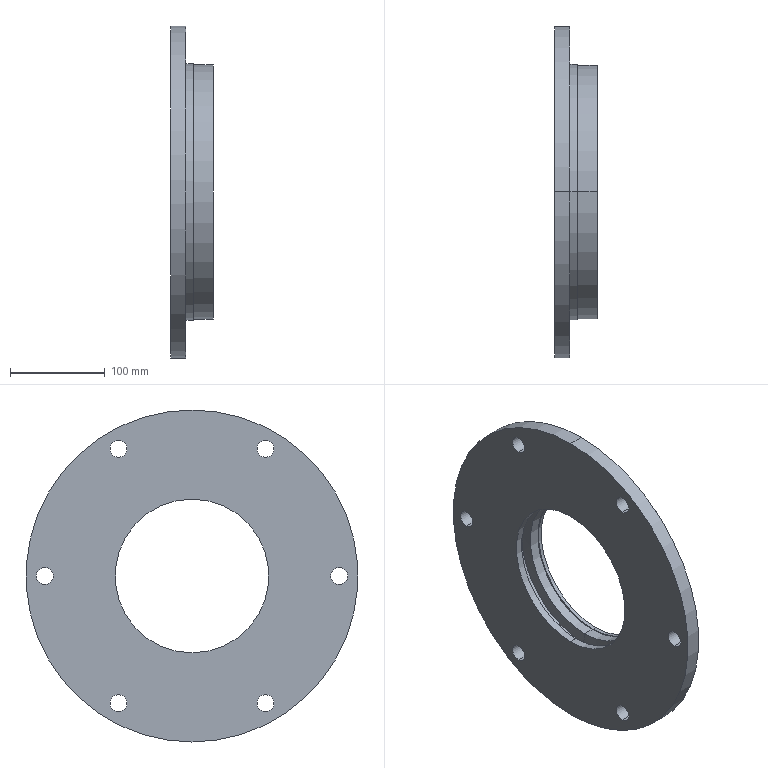Part | NX | features BREP 1 | 1 solid | 41 faces | box 45 x 350 x 350 mm | volume 1928848 mm3 | cylinder 30 | plane 7 | cone 4 | commonest cylinder face diameters 18 x12 162 x6 170 x2 185 x2 250 x2 268 x2
STEP:
#1=CARTESIAN_POINT('',(16.,77.5,-143.234));
#2=VERTEX_POINT('',#1);
#3=CARTESIAN_POINT('',(16.,77.5,-125.234));
#4=VERTEX_POINT('',#3);
#5=CARTESIAN_POINT('',(16.,77.5,-134.234));
#6=DIRECTION('',(-1.,0.,0.));
#7=DIRECTION('',(0.,0.,1.));
#8=AXIS2_PLACEMENT_3D('',#5,#6,#7);
#9=CIRCLE('',#8,9.);
#10=EDGE_CURVE('',#2,#4,#9,.T.);
#11=ORIENTED_EDGE('',*,*,#10,.F.);
#12=CARTESIAN_POINT('',(0.,77.5,-143.234));
#13=VERTEX_POINT('',#12);
#14=CARTESIAN_POINT('',(45.,77.5,-143.234));
#15=DIRECTION('',(-1.,0.,0.));
#16=VECTOR('',#15,1000.);
#17=LINE('',#14,#16);
#18=EDGE_CURVE('',#2,#13,#17,.T.);
#19=ORIENTED_EDGE('',*,*,#18,.T.);
#20=CARTESIAN_POINT('',(0.,77.5,-125.234));
#21=VERTEX_POINT('',#20);
#22=CARTESIAN_POINT('',(0.,77.5,-134.234));
#23=DIRECTION('',(-1.,0.,0.));
#24=DIRECTION('',(0.,0.866,0.5));
#25=AXIS2_PLACEMENT_3D('',#22,#23,#24);
#26=CIRCLE('',#25,9.);
#27=EDGE_CURVE('',#13,#21,#26,.T.);
#28=ORIENTED_EDGE('',*,*,#27,.T.);
#29=CARTESIAN_POINT('',(45.,77.5,-125.234));
#30=DIRECTION('',(-1.,0.,0.));
#31=VECTOR('',#30,1000.);
#32=LINE('',#29,#31);
#33=EDGE_CURVE('',#4,#21,#32,.T.);
#34=ORIENTED_EDGE('',*,*,#33,.F.);
#35=EDGE_LOOP('',(#11,#19,#28,#34));
#36=FACE_BOUND('',#35,.T.);
#37=CARTESIAN_POINT('',(45.,77.5,-134.234));
#38=DIRECTION('',(-1.,0.,0.));
#39=DIRECTION('',(0.,0.,-1.));
#40=AXIS2_PLACEMENT_3D('',#37,#38,#39);
#41=CYLINDRICAL_SURFACE('',#40,9.);
#42=ADVANCED_FACE('',(#36),#41,.F.);
#43=CARTESIAN_POINT('',(16.,-77.5,-143.234));
#44=VERTEX_POINT('',#43);
#45=CARTESIAN_POINT('',(16.,-77.5,-125.234));
#46=VERTEX_POINT('',#45);
#47=CARTESIAN_POINT('',(16.,-77.5,-134.234));
#48=DIRECTION('',(-1.,0.,0.));
#49=DIRECTION('',(0.,0.,1.));
#50=AXIS2_PLACEMENT_3D('',#47,#48,#49);
#51=CIRCLE('',#50,9.);
#52=EDGE_CURVE('',#44,#46,#51,.T.);
#53=ORIENTED_EDGE('',*,*,#52,.F.);
#54=CARTESIAN_POINT('',(0.,-77.5,-143.234));
#55=VERTEX_POINT('',#54);
#56=CARTESIAN_POINT('',(45.,-77.5,-143.234));
#57=DIRECTION('',(-1.,0.,0.));
#58=VECTOR('',#57,1000.);
#59=LINE('',#56,#58);
#60=EDGE_CURVE('',#44,#55,#59,.T.);
#61=ORIENTED_EDGE('',*,*,#60,.T.);
#62=CARTESIAN_POINT('',(0.,-77.5,-125.234));
#63=VERTEX_POINT('',#62);
#64=CARTESIAN_POINT('',(0.,-77.5,-134.234));
#65=DIRECTION('',(-1.,0.,0.));
#66=DIRECTION('',(0.,0.866,-0.5));
#67=AXIS2_PLACEMENT_3D('',#64,#65,#66);
#68=CIRCLE('',#67,9.);
#69=EDGE_CURVE('',#55,#63,#68,.T.);
#70=ORIENTED_EDGE('',*,*,#69,.T.);
#71=CARTESIAN_POINT('',(45.,-77.5,-125.234));
#72=DIRECTION('',(-1.,0.,0.));
#73=VECTOR('',#72,1000.);
#74=LINE('',#71,#73);
#75=EDGE_CURVE('',#46,#63,#74,.T.);
#76=ORIENTED_EDGE('',*,*,#75,.F.);
#77=EDGE_LOOP('',(#53,#61,#70,#76));
#78=FACE_BOUND('',#77,.T.);
#79=CARTESIAN_POINT('',(45.,-77.5,-134.234));
#80=DIRECTION('',(-1.,0.,0.));
#81=DIRECTION('',(0.,0.,-1.));
#82=AXIS2_PLACEMENT_3D('',#79,#80,#81);
#83=CYLINDRICAL_SURFACE('',#82,9.);
#84=ADVANCED_FACE('',(#78),#83,.F.);
#85=CARTESIAN_POINT('',(16.,-155.,-9.));
#86=VERTEX_POINT('',#85);
#87=CARTESIAN_POINT('',(16.,-155.,9.));
#88=VERTEX_POINT('',#87);
#89=CARTESIAN_POINT('',(16.,-155.,0.));
#90=DIRECTION('',(-1.,0.,0.));
#91=DIRECTION('',(0.,0.,1.));
#92=AXIS2_PLACEMENT_3D('',#89,#90,#91);
#93=CIRCLE('',#92,9.);
#94=EDGE_CURVE('',#86,#88,#93,.T.);
#95=ORIENTED_EDGE('',*,*,#94,.F.);
#96=CARTESIAN_POINT('',(0.,-155.,-9.));
#97=VERTEX_POINT('',#96);
#98=CARTESIAN_POINT('',(45.,-155.,-9.));
#99=DIRECTION('',(-1.,0.,0.));
#100=VECTOR('',#99,1000.);
#101=LINE('',#98,#100);
#102=EDGE_CURVE('',#86,#97,#101,.T.);
#103=ORIENTED_EDGE('',*,*,#102,.T.);
#104=CARTESIAN_POINT('',(0.,-155.,9.));
#105=VERTEX_POINT('',#104);
#106=CARTESIAN_POINT('',(0.,-155.,0.));
#107=DIRECTION('',(-1.,0.,0.));
#108=DIRECTION('',(0.,0.,-1.));
#109=AXIS2_PLACEMENT_3D('',#106,#107,#108);
#110=CIRCLE('',#109,9.);
#111=EDGE_CURVE('',#97,#105,#110,.T.);
#112=ORIENTED_EDGE('',*,*,#111,.T.);
#113=CARTESIAN_POINT('',(45.,-155.,9.));
#114=DIRECTION('',(-1.,0.,0.));
#115=VECTOR('',#114,1000.);
#116=LINE('',#113,#115);
#117=EDGE_CURVE('',#88,#105,#116,.T.);
#118=ORIENTED_EDGE('',*,*,#117,.F.);
#119=EDGE_LOOP('',(#95,#103,#112,#118));
#120=FACE_BOUND('',#119,.T.);
#121=CARTESIAN_POINT('',(45.,-155.,0.));
#122=DIRECTION('',(-1.,0.,0.));
#123=DIRECTION('',(0.,0.,-1.));
#124=AXIS2_PLACEMENT_3D('',#121,#122,#123);
#125=CYLINDRICAL_SURFACE('',#124,9.);
#126=ADVANCED_FACE('',(#120),#125,.F.);
#127=CARTESIAN_POINT('',(16.,-77.5,125.234));
#128=VERTEX_POINT('',#127);
#129=CARTESIAN_POINT('',(16.,-77.5,143.234));
#130=VERTEX_POINT('',#129);
#131=CARTESIAN_POINT('',(16.,-77.5,134.234));
#132=DIRECTION('',(-1.,0.,0.));
#133=DIRECTION('',(0.,0.,1.));
#134=AXIS2_PLACEMENT_3D('',#131,#132,#133);
#135=CIRCLE('',#134,9.);
#136=EDGE_CURVE('',#128,#130,#135,.T.);
#137=ORIENTED_EDGE('',*,*,#136,.F.);
#138=CARTESIAN_POINT('',(0.,-77.5,125.234));
#139=VERTEX_POINT('',#138);
#140=CARTESIAN_POINT('',(45.,-77.5,125.234));
#141=DIRECTION('',(-1.,0.,0.));
#142=VECTOR('',#141,1000.);
#143=LINE('',#140,#142);
#144=EDGE_CURVE('',#128,#139,#143,.T.);
#145=ORIENTED_EDGE('',*,*,#144,.T.);
#146=CARTESIAN_POINT('',(0.,-77.5,143.234));
#147=VERTEX_POINT('',#146);
#148=CARTESIAN_POINT('',(0.,-77.5,134.234));
#149=DIRECTION('',(-1.,0.,0.));
#150=DIRECTION('',(0.,-0.866,-0.5));
#151=AXIS2_PLACEMENT_3D('',#148,#149,#150);
#152=CIRCLE('',#151,9.);
#153=EDGE_CURVE('',#139,#147,#152,.T.);
#154=ORIENTED_EDGE('',*,*,#153,.T.);
#155=CARTESIAN_POINT('',(45.,-77.5,143.234));
#156=DIRECTION('',(-1.,0.,0.));
#157=VECTOR('',#156,1000.);
#158=LINE('',#155,#157);
#159=EDGE_CURVE('',#130,#147,#158,.T.);
#160=ORIENTED_EDGE('',*,*,#159,.F.);
#161=EDGE_LOOP('',(#137,#145,#154,#160));
#162=FACE_BOUND('',#161,.T.);
#163=CARTESIAN_POINT('',(45.,-77.5,134.234));
#164=DIRECTION('',(-1.,0.,0.));
#165=DIRECTION('',(0.,0.,-1.));
#166=AXIS2_PLACEMENT_3D('',#163,#164,#165);
#167=CYLINDRICAL_SURFACE('',#166,9.);
#168=ADVANCED_FACE('',(#162),#167,.F.);
#169=CARTESIAN_POINT('',(16.,77.5,125.234));
#170=VERTEX_POINT('',#169);
#171=CARTESIAN_POINT('',(16.,77.5,143.234));
#172=VERTEX_POINT('',#171);
#173=CARTESIAN_POINT('',(16.,77.5,134.234));
#174=DIRECTION('',(-1.,0.,0.));
#175=DIRECTION('',(0.,0.,1.));
#176=AXIS2_PLACEMENT_3D('',#173,#174,#175);
#177=CIRCLE('',#176,9.);
#178=EDGE_CURVE('',#170,#172,#177,.T.);
#179=ORIENTED_EDGE('',*,*,#178,.F.);
#180=CARTESIAN_POINT('',(0.,77.5,125.234));
#181=VERTEX_POINT('',#180);
#182=CARTESIAN_POINT('',(45.,77.5,125.234));
#183=DIRECTION('',(-1.,0.,0.));
#184=VECTOR('',#183,1000.);
#185=LINE('',#182,#184);
#186=EDGE_CURVE('',#170,#181,#185,.T.);
#187=ORIENTED_EDGE('',*,*,#186,.T.);
#188=CARTESIAN_POINT('',(0.,77.5,143.234));
#189=VERTEX_POINT('',#188);
#190=CARTESIAN_POINT('',(0.,77.5,134.234));
#191=DIRECTION('',(-1.,0.,0.));
#192=DIRECTION('',(0.,-0.866,0.5));
#193=AXIS2_PLACEMENT_3D('',#190,#191,#192);
#194=CIRCLE('',#193,9.);
#195=EDGE_CURVE('',#181,#189,#194,.T.);
#196=ORIENTED_EDGE('',*,*,#195,.T.);
#197=CARTESIAN_POINT('',(45.,77.5,143.234));
#198=DIRECTION('',(-1.,0.,0.));
#199=VECTOR('',#198,1000.);
#200=LINE('',#197,#199);
#201=EDGE_CURVE('',#172,#189,#200,.T.);
#202=ORIENTED_EDGE('',*,*,#201,.F.);
#203=EDGE_LOOP('',(#179,#187,#196,#202));
#204=FACE_BOUND('',#203,.T.);
#205=CARTESIAN_POINT('',(45.,77.5,134.234));
#206=DIRECTION('',(-1.,0.,0.));
#207=DIRECTION('',(0.,0.,-1.));
#208=AXIS2_PLACEMENT_3D('',#205,#206,#207);
#209=CYLINDRICAL_SURFACE('',#208,9.);
#210=ADVANCED_FACE('',(#204),#209,.F.);
#211=CARTESIAN_POINT('',(16.,155.,-9.));
#212=VERTEX_POINT('',#211);
#213=CARTESIAN_POINT('',(16.,155.,9.));
#214=VERTEX_POINT('',#213);
#215=CARTESIAN_POINT('',(16.,155.,0.));
#216=DIRECTION('',(-1.,0.,0.));
#217=DIRECTION('',(0.,0.,1.));
#218=AXIS2_PLACEMENT_3D('',#215,#216,#217);
#219=CIRCLE('',#218,9.);
#220=EDGE_CURVE('',#212,#214,#219,.T.);
#221=ORIENTED_EDGE('',*,*,#220,.F.);
#222=CARTESIAN_POINT('',(0.,155.,-9.));
#223=VERTEX_POINT('',#222);
#224=CARTESIAN_POINT('',(45.,155.,-9.));
#225=DIRECTION('',(-1.,0.,0.));
#226=VECTOR('',#225,1000.);
#227=LINE('',#224,#226);
#228=EDGE_CURVE('',#212,#223,#227,.T.);
#229=ORIENTED_EDGE('',*,*,#228,.T.);
#230=CARTESIAN_POINT('',(0.,155.,9.));
#231=VERTEX_POINT('',#230);
#232=CARTESIAN_POINT('',(0.,155.,0.));
#233=DIRECTION('',(-1.,0.,0.));
#234=DIRECTION('',(0.,0.,1.));
#235=AXIS2_PLACEMENT_3D('',#232,#233,#234);
#236=CIRCLE('',#235,9.);
#237=EDGE_CURVE('',#223,#231,#236,.T.);
#238=ORIENTED_EDGE('',*,*,#237,.T.);
#239=CARTESIAN_POINT('',(45.,155.,9.));
#240=DIRECTION('',(-1.,0.,0.));
#241=VECTOR('',#240,1000.);
#242=LINE('',#239,#241);
#243=EDGE_CURVE('',#214,#231,#242,.T.);
#244=ORIENTED_EDGE('',*,*,#243,.F.);
#245=EDGE_LOOP('',(#221,#229,#238,#244));
#246=FACE_BOUND('',#245,.T.);
#247=CARTESIAN_POINT('',(45.,155.,0.));
#248=DIRECTION('',(-1.,0.,0.));
#249=DIRECTION('',(0.,0.,-1.));
#250=AXIS2_PLACEMENT_3D('',#247,#248,#249);
#251=CYLINDRICAL_SURFACE('',#250,9.);
#252=ADVANCED_FACE('',(#246),#251,.F.);
#253=CARTESIAN_POINT('',(8.,0.,-81.));
#254=VERTEX_POINT('',#253);
#255=CARTESIAN_POINT('',(8.,0.,81.));
#256=VERTEX_POINT('',#255);
#257=CARTESIAN_POINT('',(8.,0.,0.));
#258=DIRECTION('',(-1.,0.,0.));
#259=DIRECTION('',(0.,0.,1.));
#260=AXIS2_PLACEMENT_3D('',#257,#258,#259);
#261=CIRCLE('',#260,81.);
#262=EDGE_CURVE('',#254,#256,#261,.T.);
#263=ORIENTED_EDGE('',*,*,#262,.T.);
#264=CARTESIAN_POINT('',(9.412,0.,92.5));
#265=VERTEX_POINT('',#264);
#266=CARTESIAN_POINT('',(8.,0.,81.));
#267=DIRECTION('',(0.1219,0.,0.9925));
#268=VECTOR('',#267,1000.);
#269=LINE('',#266,#268);
#270=EDGE_CURVE('',#265,#256,#269,.F.);
#271=ORIENTED_EDGE('',*,*,#270,.F.);
#272=CARTESIAN_POINT('',(9.412,0.,-92.5));
#273=VERTEX_POINT('',#272);
#274=CARTESIAN_POINT('',(9.412,0.,0.));
#275=DIRECTION('',(-1.,0.,0.));
#276=DIRECTION('',(0.,0.,1.));
#277=AXIS2_PLACEMENT_3D('',#274,#275,#276);
#278=CIRCLE('',#277,92.5);
#279=EDGE_CURVE('',#273,#265,#278,.T.);
#280=ORIENTED_EDGE('',*,*,#279,.F.);
#281=CARTESIAN_POINT('',(8.,0.,-81.));
#282=DIRECTION('',(0.1219,0.,-0.9925));
#283=VECTOR('',#282,1000.);
#284=LINE('',#281,#283);
#285=EDGE_CURVE('',#273,#254,#284,.F.);
#286=ORIENTED_EDGE('',*,*,#285,.T.);
#287=EDGE_LOOP('',(#263,#271,#280,#286));
#288=FACE_BOUND('',#287,.T.);
#289=CARTESIAN_POINT('',(8.,0.,0.));
#290=DIRECTION('',(1.,0.,0.));
#291=DIRECTION('',(0.,0.,1.));
#292=AXIS2_PLACEMENT_3D('',#289,#290,#291);
#293=CONICAL_SURFACE('',#292,81.,1.449);
#294=ADVANCED_FACE('',(#288),#293,.F.);
#295=CARTESIAN_POINT('',(19.412,0.,-92.5));
#296=VERTEX_POINT('',#295);
#297=CARTESIAN_POINT('',(19.412,0.,92.5));
#298=VERTEX_POINT('',#297);
#299=CARTESIAN_POINT('',(19.412,0.,0.));
#300=DIRECTION('',(-1.,0.,0.));
#301=DIRECTION('',(0.,0.,1.));
#302=AXIS2_PLACEMENT_3D('',#299,#300,#301);
#303=CIRCLE('',#302,92.5);
#304=EDGE_CURVE('',#296,#298,#303,.T.);
#305=ORIENTED_EDGE('',*,*,#304,.F.);
#306=CARTESIAN_POINT('',(0.,0.,-92.5));
#307=DIRECTION('',(-1.,0.,0.));
#308=VECTOR('',#307,1000.);
#309=LINE('',#306,#308);
#310=EDGE_CURVE('',#296,#273,#309,.T.);
#311=ORIENTED_EDGE('',*,*,#310,.T.);
#312=ORIENTED_EDGE('',*,*,#279,.T.);
#313=CARTESIAN_POINT('',(0.,0.,92.5));
#314=DIRECTION('',(-1.,0.,0.));
#315=VECTOR('',#314,1000.);
#316=LINE('',#313,#315);
#317=EDGE_CURVE('',#298,#265,#316,.T.);
#318=ORIENTED_EDGE('',*,*,#317,.F.);
#319=EDGE_LOOP('',(#305,#311,#312,#318));
#320=FACE_BOUND('',#319,.T.);
#321=CARTESIAN_POINT('',(0.,0.,0.));
#322=DIRECTION('',(-1.,0.,0.));
#323=DIRECTION('',(0.,0.,-1.));
#324=AXIS2_PLACEMENT_3D('',#321,#322,#323);
#325=CYLINDRICAL_SURFACE('',#324,92.5);
#326=ADVANCED_FACE('',(#320),#325,.F.);
#327=CARTESIAN_POINT('',(20.824,0.,-81.));
#328=VERTEX_POINT('',#327);
#329=CARTESIAN_POINT('',(20.824,0.,81.));
#330=VERTEX_POINT('',#329);
#331=CARTESIAN_POINT('',(20.824,0.,0.));
#332=DIRECTION('',(-1.,0.,0.));
#333=DIRECTION('',(0.,0.,1.));
#334=AXIS2_PLACEMENT_3D('',#331,#332,#333);
#335=CIRCLE('',#334,81.);
#336=EDGE_CURVE('',#328,#330,#335,.T.);
#337=ORIENTED_EDGE('',*,*,#336,.F.);
#338=CARTESIAN_POINT('',(19.412,0.,-92.5));
#339=DIRECTION('',(-0.1219,0.,-0.9925));
#340=VECTOR('',#339,1000.);
#341=LINE('',#338,#340);
#342=EDGE_CURVE('',#328,#296,#341,.T.);
#343=ORIENTED_EDGE('',*,*,#342,.T.);
#344=ORIENTED_EDGE('',*,*,#304,.T.);
#345=CARTESIAN_POINT('',(19.412,0.,92.5));
#346=DIRECTION('',(-0.1219,0.,0.9925));
#347=VECTOR('',#346,1000.);
#348=LINE('',#345,#347);
#349=EDGE_CURVE('',#330,#298,#348,.T.);
#350=ORIENTED_EDGE('',*,*,#349,.F.);
#351=EDGE_LOOP('',(#337,#343,#344,#350));
#352=FACE_BOUND('',#351,.T.);
#353=CARTESIAN_POINT('',(19.412,0.,0.));
#354=DIRECTION('',(-1.,0.,0.));
#355=DIRECTION('',(0.,0.,-1.));
#356=AXIS2_PLACEMENT_3D('',#353,#354,#355);
#357=CONICAL_SURFACE('',#356,92.5,1.449);
#358=ADVANCED_FACE('',(#352),#357,.F.);
#359=CARTESIAN_POINT('',(32.,0.,-81.));
#360=VERTEX_POINT('',#359);
#361=CARTESIAN_POINT('',(32.,0.,81.));
#362=VERTEX_POINT('',#361);
#363=CARTESIAN_POINT('',(32.,0.,0.));
#364=DIRECTION('',(-1.,0.,0.));
#365=DIRECTION('',(0.,0.,1.));
#366=AXIS2_PLACEMENT_3D('',#363,#364,#365);
#367=CIRCLE('',#366,81.);
#368=EDGE_CURVE('',#360,#362,#367,.T.);
#369=ORIENTED_EDGE('',*,*,#368,.F.);
#370=CARTESIAN_POINT('',(0.,0.,-81.));
#371=DIRECTION('',(-1.,0.,0.));
#372=VECTOR('',#371,1000.);
#373=LINE('',#370,#372);
#374=EDGE_CURVE('',#360,#328,#373,.T.);
#375=ORIENTED_EDGE('',*,*,#374,.T.);
#376=ORIENTED_EDGE('',*,*,#336,.T.);
#377=CARTESIAN_POINT('',(0.,0.,81.));
#378=DIRECTION('',(-1.,0.,0.));
#379=VECTOR('',#378,1000.);
#380=LINE('',#377,#379);
#381=EDGE_CURVE('',#362,#330,#380,.T.);
#382=ORIENTED_EDGE('',*,*,#381,.F.);
#383=EDGE_LOOP('',(#369,#375,#376,#382));
#384=FACE_BOUND('',#383,.T.);
#385=CARTESIAN_POINT('',(0.,0.,0.));
#386=DIRECTION('',(-1.,0.,0.));
#387=DIRECTION('',(0.,0.,-1.));
#388=AXIS2_PLACEMENT_3D('',#385,#386,#387);
#389=CYLINDRICAL_SURFACE('',#388,81.);
#390=ADVANCED_FACE('',(#384),#389,.F.);
#391=CARTESIAN_POINT('',(33.,0.,-85.));
#392=VERTEX_POINT('',#391);
#393=CARTESIAN_POINT('',(33.,0.,85.));
#394=VERTEX_POINT('',#393);
#395=CARTESIAN_POINT('',(33.,0.,0.));
#396=DIRECTION('',(-1.,0.,0.));
#397=DIRECTION('',(0.,0.,1.));
#398=AXIS2_PLACEMENT_3D('',#395,#396,#397);
#399=CIRCLE('',#398,85.);
#400=EDGE_CURVE('',#392,#394,#399,.T.);
#401=ORIENTED_EDGE('',*,*,#400,.F.);
#402=CARTESIAN_POINT('',(32.,0.,-85.));
#403=VERTEX_POINT('',#402);
#404=CARTESIAN_POINT('',(0.,0.,-85.));
#405=DIRECTION('',(-1.,0.,0.));
#406=VECTOR('',#405,1000.);
#407=LINE('',#404,#406);
#408=EDGE_CURVE('',#392,#403,#407,.T.);
#409=ORIENTED_EDGE('',*,*,#408,.T.);
#410=CARTESIAN_POINT('',(32.,0.,85.));
#411=VERTEX_POINT('',#410);
#412=CARTESIAN_POINT('',(32.,0.,0.));
#413=DIRECTION('',(-1.,0.,0.));
#414=DIRECTION('',(0.,0.,1.));
#415=AXIS2_PLACEMENT_3D('',#412,#413,#414);
#416=CIRCLE('',#415,85.);
#417=EDGE_CURVE('',#403,#411,#416,.T.);
#418=ORIENTED_EDGE('',*,*,#417,.T.);
#419=CARTESIAN_POINT('',(0.,0.,85.));
#420=DIRECTION('',(-1.,0.,0.));
#421=VECTOR('',#420,1000.);
#422=LINE('',#419,#421);
#423=EDGE_CURVE('',#394,#411,#422,.T.);
#424=ORIENTED_EDGE('',*,*,#423,.F.);
#425=EDGE_LOOP('',(#401,#409,#418,#424));
#426=FACE_BOUND('',#425,.T.);
#427=CARTESIAN_POINT('',(0.,0.,0.));
#428=DIRECTION('',(-1.,0.,0.));
#429=DIRECTION('',(0.,0.,-1.));
#430=AXIS2_PLACEMENT_3D('',#427,#428,#429);
#431=CYLINDRICAL_SURFACE('',#430,85.);
#432=ADVANCED_FACE('',(#426),#431,.F.);
#433=CARTESIAN_POINT('',(37.,0.,-81.));
#434=VERTEX_POINT('',#433);
#435=CARTESIAN_POINT('',(37.,0.,81.));
#436=VERTEX_POINT('',#435);
#437=CARTESIAN_POINT('',(37.,0.,0.));
#438=DIRECTION('',(-1.,0.,0.));
#439=DIRECTION('',(0.,0.,1.));
#440=AXIS2_PLACEMENT_3D('',#437,#438,#439);
#441=CIRCLE('',#440,81.);
#442=EDGE_CURVE('',#434,#436,#441,.T.);
#443=ORIENTED_EDGE('',*,*,#442,.F.);
#444=CARTESIAN_POINT('',(33.,0.,-81.));
#445=VERTEX_POINT('',#444);
#446=CARTESIAN_POINT('',(0.,0.,-81.));
#447=DIRECTION('',(-1.,0.,0.));
#448=VECTOR('',#447,1000.);
#449=LINE('',#446,#448);
#450=EDGE_CURVE('',#434,#445,#449,.T.);
#451=ORIENTED_EDGE('',*,*,#450,.T.);
#452=CARTESIAN_POINT('',(33.,0.,81.));
#453=VERTEX_POINT('',#452);
#454=CARTESIAN_POINT('',(33.,0.,0.));
#455=DIRECTION('',(-1.,0.,0.));
#456=DIRECTION('',(0.,0.,1.));
#457=AXIS2_PLACEMENT_3D('',#454,#455,#456);
#458=CIRCLE('',#457,81.);
#459=EDGE_CURVE('',#445,#453,#458,.T.);
#460=ORIENTED_EDGE('',*,*,#459,.T.);
#461=CARTESIAN_POINT('',(0.,0.,81.));
#462=DIRECTION('',(-1.,0.,0.));
#463=VECTOR('',#462,1000.);
#464=LINE('',#461,#463);
#465=EDGE_CURVE('',#436,#453,#464,.T.);
#466=ORIENTED_EDGE('',*,*,#465,.F.);
#467=EDGE_LOOP('',(#443,#451,#460,#466));
#468=FACE_BOUND('',#467,.T.);
#469=CARTESIAN_POINT('',(0.,0.,0.));
#470=DIRECTION('',(-1.,0.,0.));
#471=DIRECTION('',(0.,0.,-1.));
#472=AXIS2_PLACEMENT_3D('',#469,#470,#471);
#473=CYLINDRICAL_SURFACE('',#472,81.);
#474=ADVANCED_FACE('',(#468),#473,.F.);
#475=CARTESIAN_POINT('',(45.,0.,-125.));
#476=VERTEX_POINT('',#475);
#477=CARTESIAN_POINT('',(45.,0.,125.));
#478=VERTEX_POINT('',#477);
#479=CARTESIAN_POINT('',(45.,0.,0.));
#480=DIRECTION('',(-1.,0.,0.));
#481=DIRECTION('',(0.,0.,1.));
#482=AXIS2_PLACEMENT_3D('',#479,#480,#481);
#483=CIRCLE('',#482,125.);
#484=EDGE_CURVE('',#476,#478,#483,.T.);
#485=ORIENTED_EDGE('',*,*,#484,.F.);
#486=CARTESIAN_POINT('',(37.,0.,-125.));
#487=VERTEX_POINT('',#486);
#488=CARTESIAN_POINT('',(0.,0.,-125.));
#489=DIRECTION('',(-1.,0.,0.));
#490=VECTOR('',#489,1000.);
#491=LINE('',#488,#490);
#492=EDGE_CURVE('',#476,#487,#491,.T.);
#493=ORIENTED_EDGE('',*,*,#492,.T.);
#494=CARTESIAN_POINT('',(37.,0.,125.));
#495=VERTEX_POINT('',#494);
#496=CARTESIAN_POINT('',(37.,0.,0.));
#497=DIRECTION('',(-1.,0.,0.));
#498=DIRECTION('',(0.,0.,1.));
#499=AXIS2_PLACEMENT_3D('',#496,#497,#498);
#500=CIRCLE('',#499,125.);
#501=EDGE_CURVE('',#487,#495,#500,.T.);
#502=ORIENTED_EDGE('',*,*,#501,.T.);
#503=CARTESIAN_POINT('',(0.,0.,125.));
#504=DIRECTION('',(-1.,0.,0.));
#505=VECTOR('',#504,1000.);
#506=LINE('',#503,#505);
#507=EDGE_CURVE('',#478,#495,#506,.T.);
#508=ORIENTED_EDGE('',*,*,#507,.F.);
#509=EDGE_LOOP('',(#485,#493,#502,#508));
#510=FACE_BOUND('',#509,.T.);
#511=CARTESIAN_POINT('',(0.,0.,0.));
#512=DIRECTION('',(-1.,0.,0.));
#513=DIRECTION('',(0.,0.,-1.));
#514=AXIS2_PLACEMENT_3D('',#511,#512,#513);
#515=CYLINDRICAL_SURFACE('',#514,125.);
#516=ADVANCED_FACE('',(#510),#515,.F.);
#517=CARTESIAN_POINT('',(45.,0.,134.));
#518=VERTEX_POINT('',#517);
#519=CARTESIAN_POINT('',(45.,0.,-134.));
#520=VERTEX_POINT('',#519);
#521=CARTESIAN_POINT('',(45.,0.,0.));
#522=DIRECTION('',(-1.,0.,0.));
#523=DIRECTION('',(0.,0.,1.));
#524=AXIS2_PLACEMENT_3D('',#521,#522,#523);
#525=CIRCLE('',#524,134.);
#526=EDGE_CURVE('',#518,#520,#525,.T.);
#527=ORIENTED_EDGE('',*,*,#526,.T.);
#528=CARTESIAN_POINT('',(24.,0.,-134.));
#529=VERTEX_POINT('',#528);
#530=CARTESIAN_POINT('',(0.,0.,-134.));
#531=DIRECTION('',(-1.,0.,0.));
#532=VECTOR('',#531,1000.);
#533=LINE('',#530,#532);
#534=EDGE_CURVE('',#520,#529,#533,.T.);
#535=ORIENTED_EDGE('',*,*,#534,.T.);
#536=CARTESIAN_POINT('',(24.,0.,134.));
#537=VERTEX_POINT('',#536);
#538=CARTESIAN_POINT('',(24.,0.,0.));
#539=DIRECTION('',(-1.,0.,0.));
#540=DIRECTION('',(0.,0.,1.));
#541=AXIS2_PLACEMENT_3D('',#538,#539,#540);
#542=CIRCLE('',#541,134.);
#543=EDGE_CURVE('',#537,#529,#542,.T.);
#544=ORIENTED_EDGE('',*,*,#543,.F.);
#545=CARTESIAN_POINT('',(0.,0.,134.));
#546=DIRECTION('',(-1.,0.,0.));
#547=VECTOR('',#546,1000.);
#548=LINE('',#545,#547);
#549=EDGE_CURVE('',#518,#537,#548,.T.);
#550=ORIENTED_EDGE('',*,*,#549,.F.);
#551=EDGE_LOOP('',(#527,#535,#544,#550));
#552=FACE_BOUND('',#551,.T.);
#553=CARTESIAN_POINT('',(0.,0.,0.));
#554=DIRECTION('',(-1.,0.,0.));
#555=DIRECTION('',(0.,0.,-1.));
#556=AXIS2_PLACEMENT_3D('',#553,#554,#555);
#557=CYLINDRICAL_SURFACE('',#556,134.);
#558=ADVANCED_FACE('',(#552),#557,.T.);
#559=CARTESIAN_POINT('',(24.,0.,135.));
#560=VERTEX_POINT('',#559);
#561=CARTESIAN_POINT('',(24.,0.,-135.));
#562=VERTEX_POINT('',#561);
#563=CARTESIAN_POINT('',(24.,0.,0.));
#564=DIRECTION('',(-1.,0.,0.));
#565=DIRECTION('',(0.,0.,1.));
#566=AXIS2_PLACEMENT_3D('',#563,#564,#565);
#567=CIRCLE('',#566,135.);
#568=EDGE_CURVE('',#560,#562,#567,.T.);
#569=ORIENTED_EDGE('',*,*,#568,.T.);
#570=CARTESIAN_POINT('',(16.,0.,-135.));
#571=VERTEX_POINT('',#570);
#572=CARTESIAN_POINT('',(0.,0.,-135.));
#573=DIRECTION('',(-1.,0.,0.));
#574=VECTOR('',#573,1000.);
#575=LINE('',#572,#574);
#576=EDGE_CURVE('',#562,#571,#575,.T.);
#577=ORIENTED_EDGE('',*,*,#576,.T.);
#578=CARTESIAN_POINT('',(16.,0.,135.));
#579=VERTEX_POINT('',#578);
#580=CARTESIAN_POINT('',(16.,0.,0.));
#581=DIRECTION('',(-1.,0.,0.));
#582=DIRECTION('',(0.,0.,1.));
#583=AXIS2_PLACEMENT_3D('',#580,#581,#582);
#584=CIRCLE('',#583,135.);
#585=EDGE_CURVE('',#579,#571,#584,.T.);
#586=ORIENTED_EDGE('',*,*,#585,.F.);
#587=CARTESIAN_POINT('',(0.,0.,135.));
#588=DIRECTION('',(-1.,0.,0.));
#589=VECTOR('',#588,1000.);
#590=LINE('',#587,#589);
#591=EDGE_CURVE('',#560,#579,#590,.T.);
#592=ORIENTED_EDGE('',*,*,#591,.F.);
#593=EDGE_LOOP('',(#569,#577,#586,#592));
#594=FACE_BOUND('',#593,.T.);
#595=CARTESIAN_POINT('',(0.,0.,0.));
#596=DIRECTION('',(-1.,0.,0.));
#597=DIRECTION('',(0.,0.,-1.));
#598=AXIS2_PLACEMENT_3D('',#595,#596,#597);
#599=CYLINDRICAL_SURFACE('',#598,135.);
#600=ADVANCED_FACE('',(#594),#599,.T.);
#601=CARTESIAN_POINT('',(16.,0.,175.));
#602=VERTEX_POINT('',#601);
#603=CARTESIAN_POINT('',(16.,0.,-175.));
#604=VERTEX_POINT('',#603);
#605=CARTESIAN_POINT('',(16.,0.,0.));
#606=DIRECTION('',(-1.,0.,0.));
#607=DIRECTION('',(0.,0.,1.));
#608=AXIS2_PLACEMENT_3D('',#605,#606,#607);
#609=CIRCLE('',#608,175.);
#610=EDGE_CURVE('',#602,#604,#609,.T.);
#611=ORIENTED_EDGE('',*,*,#610,.T.);
#612=CARTESIAN_POINT('',(0.,0.,-175.));
#613=VERTEX_POINT('',#612);
#614=CARTESIAN_POINT('',(0.,0.,-175.));
#615=DIRECTION('',(-1.,0.,0.));
#616=VECTOR('',#615,1000.);
#617=LINE('',#614,#616);
#618=EDGE_CURVE('',#604,#613,#617,.T.);
#619=ORIENTED_EDGE('',*,*,#618,.T.);
#620=CARTESIAN_POINT('',(0.,0.,175.));
#621=VERTEX_POINT('',#620);
#622=CARTESIAN_POINT('',(0.,0.,0.));
#623=DIRECTION('',(-1.,0.,0.));
#624=DIRECTION('',(0.,0.,1.));
#625=AXIS2_PLACEMENT_3D('',#622,#623,#624);
#626=CIRCLE('',#625,175.);
#627=EDGE_CURVE('',#621,#613,#626,.T.);
#628=ORIENTED_EDGE('',*,*,#627,.F.);
#629=CARTESIAN_POINT('',(0.,0.,175.));
#630=DIRECTION('',(-1.,0.,0.));
#631=VECTOR('',#630,1000.);
#632=LINE('',#629,#631);
#633=EDGE_CURVE('',#602,#621,#632,.T.);
#634=ORIENTED_EDGE('',*,*,#633,.F.);
#635=EDGE_LOOP('',(#611,#619,#628,#634));
#636=FACE_BOUND('',#635,.T.);
#637=CARTESIAN_POINT('',(0.,0.,0.));
#638=DIRECTION('',(-1.,0.,0.));
#639=DIRECTION('',(0.,0.,-1.));
#640=AXIS2_PLACEMENT_3D('',#637,#638,#639);
#641=CYLINDRICAL_SURFACE('',#640,175.);
#642=ADVANCED_FACE('',(#636),#641,.T.);
#643=ORIENTED_EDGE('',*,*,#262,.F.);
#644=CARTESIAN_POINT('',(0.,0.,-81.));
#645=VERTEX_POINT('',#644);
#646=CARTESIAN_POINT('',(0.,0.,-81.));
#647=DIRECTION('',(-1.,0.,0.));
#648=VECTOR('',#647,1000.);
#649=LINE('',#646,#648);
#650=EDGE_CURVE('',#254,#645,#649,.T.);
#651=ORIENTED_EDGE('',*,*,#650,.T.);
#652=CARTESIAN_POINT('',(0.,0.,81.));
#653=VERTEX_POINT('',#652);
#654=CARTESIAN_POINT('',(0.,0.,0.));
#655=DIRECTION('',(-1.,0.,0.));
#656=DIRECTION('',(0.,0.,1.));
#657=AXIS2_PLACEMENT_3D('',#654,#655,#656);
#658=CIRCLE('',#657,81.);
#659=EDGE_CURVE('',#645,#653,#658,.T.);
#660=ORIENTED_EDGE('',*,*,#659,.T.);
#661=CARTESIAN_POINT('',(0.,0.,81.));
#662=DIRECTION('',(-1.,0.,0.));
#663=VECTOR('',#662,1000.);
#664=LINE('',#661,#663);
#665=EDGE_CURVE('',#256,#653,#664,.T.);
#666=ORIENTED_EDGE('',*,*,#665,.F.);
#667=EDGE_LOOP('',(#643,#651,#660,#666));
#668=FACE_BOUND('',#667,.T.);
#669=CARTESIAN_POINT('',(0.,0.,0.));
#670=DIRECTION('',(-1.,0.,0.));
#671=DIRECTION('',(0.,0.,-1.));
#672=AXIS2_PLACEMENT_3D('',#669,#670,#671);
#673=CYLINDRICAL_SURFACE('',#672,81.);
#674=ADVANCED_FACE('',(#668),#673,.F.);
#675=ORIENTED_EDGE('',*,*,#650,.F.);
#676=CARTESIAN_POINT('',(8.,0.,0.));
#677=DIRECTION('',(-1.,0.,0.));
#678=DIRECTION('',(0.,0.,1.));
#679=AXIS2_PLACEMENT_3D('',#676,#677,#678);
#680=CIRCLE('',#679,81.);
#681=EDGE_CURVE('',#256,#254,#680,.T.);
#682=ORIENTED_EDGE('',*,*,#681,.F.);
#683=ORIENTED_EDGE('',*,*,#665,.T.);
#684=CARTESIAN_POINT('',(0.,0.,0.));
#685=DIRECTION('',(-1.,0.,0.));
#686=DIRECTION('',(0.,0.,1.));
#687=AXIS2_PLACEMENT_3D('',#684,#685,#686);
#688=CIRCLE('',#687,81.);
#689=EDGE_CURVE('',#653,#645,#688,.T.);
#690=ORIENTED_EDGE('',*,*,#689,.T.);
#691=EDGE_LOOP('',(#675,#682,#683,#690));
#692=FACE_BOUND('',#691,.T.);
#693=CARTESIAN_POINT('',(0.,0.,0.));
#694=DIRECTION('',(-1.,0.,0.));
#695=DIRECTION('',(0.,0.,-1.));
#696=AXIS2_PLACEMENT_3D('',#693,#694,#695);
#697=CYLINDRICAL_SURFACE('',#696,81.);
#698=ADVANCED_FACE('',(#692),#697,.F.);
#699=CARTESIAN_POINT('',(0.,77.5,-134.234));
#700=DIRECTION('',(-1.,0.,0.));
#701=DIRECTION('',(0.,0.866,0.5));
#702=AXIS2_PLACEMENT_3D('',#699,#700,#701);
#703=CIRCLE('',#702,9.);
#704=EDGE_CURVE('',#21,#13,#703,.T.);
#705=ORIENTED_EDGE('',*,*,#704,.F.);
#706=ORIENTED_EDGE('',*,*,#27,.F.);
#707=EDGE_LOOP('',(#705,#706));
#708=FACE_BOUND('',#707,.T.);
#709=CARTESIAN_POINT('',(0.,-77.5,-134.234));
#710=DIRECTION('',(-1.,0.,0.));
#711=DIRECTION('',(0.,0.866,-0.5));
#712=AXIS2_PLACEMENT_3D('',#709,#710,#711);
#713=CIRCLE('',#712,9.);
#714=EDGE_CURVE('',#63,#55,#713,.T.);
#715=ORIENTED_EDGE('',*,*,#714,.F.);
#716=ORIENTED_EDGE('',*,*,#69,.F.);
#717=EDGE_LOOP('',(#715,#716));
#718=FACE_BOUND('',#717,.T.);
#719=CARTESIAN_POINT('',(0.,-155.,0.));
#720=DIRECTION('',(-1.,0.,0.));
#721=DIRECTION('',(0.,0.,-1.));
#722=AXIS2_PLACEMENT_3D('',#719,#720,#721);
#723=CIRCLE('',#722,9.);
#724=EDGE_CURVE('',#105,#97,#723,.T.);
#725=ORIENTED_EDGE('',*,*,#724,.F.);
#726=ORIENTED_EDGE('',*,*,#111,.F.);
#727=EDGE_LOOP('',(#725,#726));
#728=FACE_BOUND('',#727,.T.);
#729=CARTESIAN_POINT('',(0.,-77.5,134.234));
#730=DIRECTION('',(-1.,0.,0.));
#731=DIRECTION('',(0.,-0.866,-0.5));
#732=AXIS2_PLACEMENT_3D('',#729,#730,#731);
#733=CIRCLE('',#732,9.);
#734=EDGE_CURVE('',#147,#139,#733,.T.);
#735=ORIENTED_EDGE('',*,*,#734,.F.);
#736=ORIENTED_EDGE('',*,*,#153,.F.);
#737=EDGE_LOOP('',(#735,#736));
#738=FACE_BOUND('',#737,.T.);
#739=CARTESIAN_POINT('',(0.,77.5,134.234));
#740=DIRECTION('',(-1.,0.,0.));
#741=DIRECTION('',(0.,-0.866,0.5));
#742=AXIS2_PLACEMENT_3D('',#739,#740,#741);
#743=CIRCLE('',#742,9.);
#744=EDGE_CURVE('',#189,#181,#743,.T.);
#745=ORIENTED_EDGE('',*,*,#744,.F.);
#746=ORIENTED_EDGE('',*,*,#195,.F.);
#747=EDGE_LOOP('',(#745,#746));
#748=FACE_BOUND('',#747,.T.);
#749=CARTESIAN_POINT('',(0.,155.,0.));
#750=DIRECTION('',(-1.,0.,0.));
#751=DIRECTION('',(0.,0.,1.));
#752=AXIS2_PLACEMENT_3D('',#749,#750,#751);
#753=CIRCLE('',#752,9.);
#754=EDGE_CURVE('',#231,#223,#753,.T.);
#755=ORIENTED_EDGE('',*,*,#754,.F.);
#756=ORIENTED_EDGE('',*,*,#237,.F.);
#757=EDGE_LOOP('',(#755,#756));
#758=FACE_BOUND('',#757,.T.);
#759=ORIENTED_EDGE('',*,*,#689,.F.);
#760=ORIENTED_EDGE('',*,*,#659,.F.);
#761=EDGE_LOOP('',(#759,#760));
#762=FACE_BOUND('',#761,.T.);
#763=ORIENTED_EDGE('',*,*,#627,.T.);
#764=CARTESIAN_POINT('',(0.,0.,0.));
#765=DIRECTION('',(-1.,0.,0.));
#766=DIRECTION('',(0.,0.,1.));
#767=AXIS2_PLACEMENT_3D('',#764,#765,#766);
#768=CIRCLE('',#767,175.);
#769=EDGE_CURVE('',#613,#621,#768,.T.);
#770=ORIENTED_EDGE('',*,*,#769,.T.);
#771=EDGE_LOOP('',(#763,#770));
#772=FACE_BOUND('',#771,.T.);
#773=CARTESIAN_POINT('',(0.,81.,0.));
#774=DIRECTION('',(1.,0.,0.));
#775=DIRECTION('',(0.,0.,1.));
#776=AXIS2_PLACEMENT_3D('',#773,#774,#775);
#777=PLANE('',#776);
#778=ADVANCED_FACE('',(#708,#718,#728,#738,#748,#758,#762,#772),#777,.F.);
#779=ORIENTED_EDGE('',*,*,#618,.F.);
#780=CARTESIAN_POINT('',(16.,0.,0.));
#781=DIRECTION('',(-1.,0.,0.));
#782=DIRECTION('',(0.,0.,1.));
#783=AXIS2_PLACEMENT_3D('',#780,#781,#782);
#784=CIRCLE('',#783,175.);
#785=EDGE_CURVE('',#604,#602,#784,.T.);
#786=ORIENTED_EDGE('',*,*,#785,.T.);
#787=ORIENTED_EDGE('',*,*,#633,.T.);
#788=ORIENTED_EDGE('',*,*,#769,.F.);
#789=EDGE_LOOP('',(#779,#786,#787,#788));
#790=FACE_BOUND('',#789,.T.);
#791=CARTESIAN_POINT('',(0.,0.,0.));
#792=DIRECTION('',(-1.,0.,0.));
#793=DIRECTION('',(0.,0.,-1.));
#794=AXIS2_PLACEMENT_3D('',#791,#792,#793);
#795=CYLINDRICAL_SURFACE('',#794,175.);
#796=ADVANCED_FACE('',(#790),#795,.T.);
#797=CARTESIAN_POINT('',(16.,77.5,-134.234));
#798=DIRECTION('',(-1.,0.,0.));
#799=DIRECTION('',(0.,0.,1.));
#800=AXIS2_PLACEMENT_3D('',#797,#798,#799);
#801=CIRCLE('',#800,9.);
#802=EDGE_CURVE('',#4,#2,#801,.T.);
#803=ORIENTED_EDGE('',*,*,#802,.T.);
#804=ORIENTED_EDGE('',*,*,#10,.T.);
#805=EDGE_LOOP('',(#803,#804));
#806=FACE_BOUND('',#805,.T.);
#807=CARTESIAN_POINT('',(16.,-77.5,-134.234));
#808=DIRECTION('',(-1.,0.,0.));
#809=DIRECTION('',(0.,0.,1.));
#810=AXIS2_PLACEMENT_3D('',#807,#808,#809);
#811=CIRCLE('',#810,9.);
#812=EDGE_CURVE('',#46,#44,#811,.T.);
#813=ORIENTED_EDGE('',*,*,#812,.T.);
#814=ORIENTED_EDGE('',*,*,#52,.T.);
#815=EDGE_LOOP('',(#813,#814));
#816=FACE_BOUND('',#815,.T.);
#817=CARTESIAN_POINT('',(16.,-155.,0.));
#818=DIRECTION('',(-1.,0.,0.));
#819=DIRECTION('',(0.,0.,1.));
#820=AXIS2_PLACEMENT_3D('',#817,#818,#819);
#821=CIRCLE('',#820,9.);
#822=EDGE_CURVE('',#88,#86,#821,.T.);
#823=ORIENTED_EDGE('',*,*,#822,.T.);
#824=ORIENTED_EDGE('',*,*,#94,.T.);
#825=EDGE_LOOP('',(#823,#824));
#826=FACE_BOUND('',#825,.T.);
#827=CARTESIAN_POINT('',(16.,-77.5,134.234));
#828=DIRECTION('',(-1.,0.,0.));
#829=DIRECTION('',(0.,0.,1.));
#830=AXIS2_PLACEMENT_3D('',#827,#828,#829);
#831=CIRCLE('',#830,9.);
#832=EDGE_CURVE('',#130,#128,#831,.T.);
#833=ORIENTED_EDGE('',*,*,#832,.T.);
#834=ORIENTED_EDGE('',*,*,#136,.T.);
#835=EDGE_LOOP('',(#833,#834));
#836=FACE_BOUND('',#835,.T.);
#837=CARTESIAN_POINT('',(16.,77.5,134.234));
#838=DIRECTION('',(-1.,0.,0.));
#839=DIRECTION('',(0.,0.,1.));
#840=AXIS2_PLACEMENT_3D('',#837,#838,#839);
#841=CIRCLE('',#840,9.);
#842=EDGE_CURVE('',#172,#170,#841,.T.);
#843=ORIENTED_EDGE('',*,*,#842,.T.);
#844=ORIENTED_EDGE('',*,*,#178,.T.);
#845=EDGE_LOOP('',(#843,#844));
#846=FACE_BOUND('',#845,.T.);
#847=CARTESIAN_POINT('',(16.,155.,0.));
#848=DIRECTION('',(-1.,0.,0.));
#849=DIRECTION('',(0.,0.,1.));
#850=AXIS2_PLACEMENT_3D('',#847,#848,#849);
#851=CIRCLE('',#850,9.);
#852=EDGE_CURVE('',#214,#212,#851,.T.);
#853=ORIENTED_EDGE('',*,*,#852,.T.);
#854=ORIENTED_EDGE('',*,*,#220,.T.);
#855=EDGE_LOOP('',(#853,#854));
#856=FACE_BOUND('',#855,.T.);
#857=ORIENTED_EDGE('',*,*,#610,.F.);
#858=ORIENTED_EDGE('',*,*,#785,.F.);
#859=EDGE_LOOP('',(#857,#858));
#860=FACE_BOUND('',#859,.T.);
#861=ORIENTED_EDGE('',*,*,#585,.T.);
#862=CARTESIAN_POINT('',(16.,0.,0.));
#863=DIRECTION('',(-1.,0.,0.));
#864=DIRECTION('',(0.,0.,1.));
#865=AXIS2_PLACEMENT_3D('',#862,#863,#864);
#866=CIRCLE('',#865,135.);
#867=EDGE_CURVE('',#571,#579,#866,.T.);
#868=ORIENTED_EDGE('',*,*,#867,.T.);
#869=EDGE_LOOP('',(#861,#868));
#870=FACE_BOUND('',#869,.T.);
#871=CARTESIAN_POINT('',(16.,175.,0.));
#872=DIRECTION('',(-1.,0.,0.));
#873=DIRECTION('',(0.,0.,-1.));
#874=AXIS2_PLACEMENT_3D('',#871,#872,#873);
#875=PLANE('',#874);
#876=ADVANCED_FACE('',(#806,#816,#826,#836,#846,#856,#860,#870),#875,.F.);
#877=ORIENTED_EDGE('',*,*,#576,.F.);
#878=CARTESIAN_POINT('',(24.,0.,0.));
#879=DIRECTION('',(-1.,0.,0.));
#880=DIRECTION('',(0.,0.,1.));
#881=AXIS2_PLACEMENT_3D('',#878,#879,#880);
#882=CIRCLE('',#881,135.);
#883=EDGE_CURVE('',#562,#560,#882,.T.);
#884=ORIENTED_EDGE('',*,*,#883,.T.);
#885=ORIENTED_EDGE('',*,*,#591,.T.);
#886=ORIENTED_EDGE('',*,*,#867,.F.);
#887=EDGE_LOOP('',(#877,#884,#885,#886));
#888=FACE_BOUND('',#887,.T.);
#889=CARTESIAN_POINT('',(0.,0.,0.));
#890=DIRECTION('',(-1.,0.,0.));
#891=DIRECTION('',(0.,0.,-1.));
#892=AXIS2_PLACEMENT_3D('',#889,#890,#891);
#893=CYLINDRICAL_SURFACE('',#892,135.);
#894=ADVANCED_FACE('',(#888),#893,.T.);
#895=ORIENTED_EDGE('',*,*,#568,.F.);
#896=ORIENTED_EDGE('',*,*,#883,.F.);
#897=EDGE_LOOP('',(#895,#896));
#898=FACE_BOUND('',#897,.T.);
#899=ORIENTED_EDGE('',*,*,#543,.T.);
#900=CARTESIAN_POINT('',(24.,0.,0.));
#901=DIRECTION('',(-1.,0.,0.));
#902=DIRECTION('',(0.,0.,1.));
#903=AXIS2_PLACEMENT_3D('',#900,#901,#902);
#904=CIRCLE('',#903,134.);
#905=EDGE_CURVE('',#529,#537,#904,.T.);
#906=ORIENTED_EDGE('',*,*,#905,.T.);
#907=EDGE_LOOP('',(#899,#906));
#908=FACE_BOUND('',#907,.T.);
#909=CARTESIAN_POINT('',(24.,135.,0.));
#910=DIRECTION('',(-1.,0.,0.));
#911=DIRECTION('',(0.,0.,-1.));
#912=AXIS2_PLACEMENT_3D('',#909,#910,#911);
#913=PLANE('',#912);
#914=ADVANCED_FACE('',(#898,#908),#913,.F.);
#915=ORIENTED_EDGE('',*,*,#534,.F.);
#916=CARTESIAN_POINT('',(45.,0.,0.));
#917=DIRECTION('',(-1.,0.,0.));
#918=DIRECTION('',(0.,0.,1.));
#919=AXIS2_PLACEMENT_3D('',#916,#917,#918);
#920=CIRCLE('',#919,134.);
#921=EDGE_CURVE('',#520,#518,#920,.T.);
#922=ORIENTED_EDGE('',*,*,#921,.T.);
#923=ORIENTED_EDGE('',*,*,#549,.T.);
#924=ORIENTED_EDGE('',*,*,#905,.F.);
#925=EDGE_LOOP('',(#915,#922,#923,#924));
#926=FACE_BOUND('',#925,.T.);
#927=CARTESIAN_POINT('',(0.,0.,0.));
#928=DIRECTION('',(-1.,0.,0.));
#929=DIRECTION('',(0.,0.,-1.));
#930=AXIS2_PLACEMENT_3D('',#927,#928,#929);
#931=CYLINDRICAL_SURFACE('',#930,134.);
#932=ADVANCED_FACE('',(#926),#931,.T.);
#933=ORIENTED_EDGE('',*,*,#526,.F.);
#934=ORIENTED_EDGE('',*,*,#921,.F.);
#935=EDGE_LOOP('',(#933,#934));
#936=FACE_BOUND('',#935,.T.);
#937=CARTESIAN_POINT('',(45.,0.,0.));
#938=DIRECTION('',(-1.,0.,0.));
#939=DIRECTION('',(0.,0.,1.));
#940=AXIS2_PLACEMENT_3D('',#937,#938,#939);
#941=CIRCLE('',#940,125.);
#942=EDGE_CURVE('',#478,#476,#941,.T.);
#943=ORIENTED_EDGE('',*,*,#942,.T.);
#944=ORIENTED_EDGE('',*,*,#484,.T.);
#945=EDGE_LOOP('',(#943,#944));
#946=FACE_BOUND('',#945,.T.);
#947=CARTESIAN_POINT('',(45.,134.,0.));
#948=DIRECTION('',(-1.,0.,0.));
#949=DIRECTION('',(0.,0.,-1.));
#950=AXIS2_PLACEMENT_3D('',#947,#948,#949);
#951=PLANE('',#950);
#952=ADVANCED_FACE('',(#936,#946),#951,.F.);
#953=ORIENTED_EDGE('',*,*,#492,.F.);
#954=ORIENTED_EDGE('',*,*,#942,.F.);
#955=ORIENTED_EDGE('',*,*,#507,.T.);
#956=CARTESIAN_POINT('',(37.,0.,0.));
#957=DIRECTION('',(-1.,0.,0.));
#958=DIRECTION('',(0.,0.,1.));
#959=AXIS2_PLACEMENT_3D('',#956,#957,#958);
#960=CIRCLE('',#959,125.);
#961=EDGE_CURVE('',#495,#487,#960,.T.);
#962=ORIENTED_EDGE('',*,*,#961,.T.);
#963=EDGE_LOOP('',(#953,#954,#955,#962));
#964=FACE_BOUND('',#963,.T.);
#965=CARTESIAN_POINT('',(0.,0.,0.));
#966=DIRECTION('',(-1.,0.,0.));
#967=DIRECTION('',(0.,0.,-1.));
#968=AXIS2_PLACEMENT_3D('',#965,#966,#967);
#969=CYLINDRICAL_SURFACE('',#968,125.);
#970=ADVANCED_FACE('',(#964),#969,.F.);
#971=ORIENTED_EDGE('',*,*,#961,.F.);
#972=ORIENTED_EDGE('',*,*,#501,.F.);
#973=EDGE_LOOP('',(#971,#972));
#974=FACE_BOUND('',#973,.T.);
#975=CARTESIAN_POINT('',(37.,0.,0.));
#976=DIRECTION('',(-1.,0.,0.));
#977=DIRECTION('',(0.,0.,1.));
#978=AXIS2_PLACEMENT_3D('',#975,#976,#977);
#979=CIRCLE('',#978,81.);
#980=EDGE_CURVE('',#436,#434,#979,.T.);
#981=ORIENTED_EDGE('',*,*,#980,.T.);
#982=ORIENTED_EDGE('',*,*,#442,.T.);
#983=EDGE_LOOP('',(#981,#982));
#984=FACE_BOUND('',#983,.T.);
#985=CARTESIAN_POINT('',(37.,125.,0.));
#986=DIRECTION('',(-1.,0.,0.));
#987=DIRECTION('',(0.,0.,-1.));
#988=AXIS2_PLACEMENT_3D('',#985,#986,#987);
#989=PLANE('',#988);
#990=ADVANCED_FACE('',(#974,#984),#989,.F.);
#991=ORIENTED_EDGE('',*,*,#450,.F.);
#992=ORIENTED_EDGE('',*,*,#980,.F.);
#993=ORIENTED_EDGE('',*,*,#465,.T.);
#994=CARTESIAN_POINT('',(33.,0.,0.));
#995=DIRECTION('',(-1.,0.,0.));
#996=DIRECTION('',(0.,0.,1.));
#997=AXIS2_PLACEMENT_3D('',#994,#995,#996);
#998=CIRCLE('',#997,81.);
#999=EDGE_CURVE('',#453,#445,#998,.T.);
#1000=ORIENTED_EDGE('',*,*,#999,.T.);
#1001=EDGE_LOOP('',(#991,#992,#993,#1000));
#1002=FACE_BOUND('',#1001,.T.);
#1003=CARTESIAN_POINT('',(0.,0.,0.));
#1004=DIRECTION('',(-1.,0.,0.));
#1005=DIRECTION('',(0.,0.,-1.));
#1006=AXIS2_PLACEMENT_3D('',#1003,#1004,#1005);
#1007=CYLINDRICAL_SURFACE('',#1006,81.);
#1008=ADVANCED_FACE('',(#1002),#1007,.F.);
#1009=ORIENTED_EDGE('',*,*,#999,.F.);
#1010=ORIENTED_EDGE('',*,*,#459,.F.);
#1011=EDGE_LOOP('',(#1009,#1010));
#1012=FACE_BOUND('',#1011,.T.);
#1013=CARTESIAN_POINT('',(33.,0.,0.));
#1014=DIRECTION('',(-1.,0.,0.));
#1015=DIRECTION('',(0.,0.,1.));
#1016=AXIS2_PLACEMENT_3D('',#1013,#1014,#1015);
#1017=CIRCLE('',#1016,85.);
#1018=EDGE_CURVE('',#394,#392,#1017,.T.);
#1019=ORIENTED_EDGE('',*,*,#1018,.T.);
#1020=ORIENTED_EDGE('',*,*,#400,.T.);
#1021=EDGE_LOOP('',(#1019,#1020));
#1022=FACE_BOUND('',#1021,.T.);
#1023=CARTESIAN_POINT('',(33.,81.,0.));
#1024=DIRECTION('',(1.,0.,0.));
#1025=DIRECTION('',(0.,0.,1.));
#1026=AXIS2_PLACEMENT_3D('',#1023,#1024,#1025);
#1027=PLANE('',#1026);
#1028=ADVANCED_FACE('',(#1012,#1022),#1027,.F.);
#1029=ORIENTED_EDGE('',*,*,#408,.F.);
#1030=ORIENTED_EDGE('',*,*,#1018,.F.);
#1031=ORIENTED_EDGE('',*,*,#423,.T.);
#1032=CARTESIAN_POINT('',(32.,0.,0.));
#1033=DIRECTION('',(-1.,0.,0.));
#1034=DIRECTION('',(0.,0.,1.));
#1035=AXIS2_PLACEMENT_3D('',#1032,#1033,#1034);
#1036=CIRCLE('',#1035,85.);
#1037=EDGE_CURVE('',#411,#403,#1036,.T.);
#1038=ORIENTED_EDGE('',*,*,#1037,.T.);
#1039=EDGE_LOOP('',(#1029,#1030,#1031,#1038));
#1040=FACE_BOUND('',#1039,.T.);
#1041=CARTESIAN_POINT('',(0.,0.,0.));
#1042=DIRECTION('',(-1.,0.,0.));
#1043=DIRECTION('',(0.,0.,-1.));
#1044=AXIS2_PLACEMENT_3D('',#1041,#1042,#1043);
#1045=CYLINDRICAL_SURFACE('',#1044,85.);
#1046=ADVANCED_FACE('',(#1040),#1045,.F.);
#1047=ORIENTED_EDGE('',*,*,#1037,.F.);
#1048=ORIENTED_EDGE('',*,*,#417,.F.);
#1049=EDGE_LOOP('',(#1047,#1048));
#1050=FACE_BOUND('',#1049,.T.);
#1051=CARTESIAN_POINT('',(32.,0.,0.));
#1052=DIRECTION('',(-1.,0.,0.));
#1053=DIRECTION('',(0.,0.,1.));
#1054=AXIS2_PLACEMENT_3D('',#1051,#1052,#1053);
#1055=CIRCLE('',#1054,81.);
#1056=EDGE_CURVE('',#362,#360,#1055,.T.);
#1057=ORIENTED_EDGE('',*,*,#1056,.T.);
#1058=ORIENTED_EDGE('',*,*,#368,.T.);
#1059=EDGE_LOOP('',(#1057,#1058));
#1060=FACE_BOUND('',#1059,.T.);
#1061=CARTESIAN_POINT('',(32.,85.,0.));
#1062=DIRECTION('',(-1.,0.,0.));
#1063=DIRECTION('',(0.,0.,-1.));
#1064=AXIS2_PLACEMENT_3D('',#1061,#1062,#1063);
#1065=PLANE('',#1064);
#1066=ADVANCED_FACE('',(#1050,#1060),#1065,.F.);
#1067=ORIENTED_EDGE('',*,*,#374,.F.);
#1068=ORIENTED_EDGE('',*,*,#1056,.F.);
#1069=ORIENTED_EDGE('',*,*,#381,.T.);
#1070=CARTESIAN_POINT('',(20.824,0.,0.));
#1071=DIRECTION('',(-1.,0.,0.));
#1072=DIRECTION('',(0.,0.,1.));
#1073=AXIS2_PLACEMENT_3D('',#1070,#1071,#1072);
#1074=CIRCLE('',#1073,81.);
#1075=EDGE_CURVE('',#330,#328,#1074,.T.);
#1076=ORIENTED_EDGE('',*,*,#1075,.T.);
#1077=EDGE_LOOP('',(#1067,#1068,#1069,#1076));
#1078=FACE_BOUND('',#1077,.T.);
#1079=CARTESIAN_POINT('',(0.,0.,0.));
#1080=DIRECTION('',(-1.,0.,0.));
#1081=DIRECTION('',(0.,0.,-1.));
#1082=AXIS2_PLACEMENT_3D('',#1079,#1080,#1081);
#1083=CYLINDRICAL_SURFACE('',#1082,81.);
#1084=ADVANCED_FACE('',(#1078),#1083,.F.);
#1085=ORIENTED_EDGE('',*,*,#342,.F.);
#1086=ORIENTED_EDGE('',*,*,#1075,.F.);
#1087=ORIENTED_EDGE('',*,*,#349,.T.);
#1088=CARTESIAN_POINT('',(19.412,0.,0.));
#1089=DIRECTION('',(-1.,0.,0.));
#1090=DIRECTION('',(0.,0.,1.));
#1091=AXIS2_PLACEMENT_3D('',#1088,#1089,#1090);
#1092=CIRCLE('',#1091,92.5);
#1093=EDGE_CURVE('',#298,#296,#1092,.T.);
#1094=ORIENTED_EDGE('',*,*,#1093,.T.);
#1095=EDGE_LOOP('',(#1085,#1086,#1087,#1094));
#1096=FACE_BOUND('',#1095,.T.);
#1097=CARTESIAN_POINT('',(19.412,0.,0.));
#1098=DIRECTION('',(-1.,0.,0.));
#1099=DIRECTION('',(0.,0.,-1.));
#1100=AXIS2_PLACEMENT_3D('',#1097,#1098,#1099);
#1101=CONICAL_SURFACE('',#1100,92.5,1.449);
#1102=ADVANCED_FACE('',(#1096),#1101,.F.);
#1103=ORIENTED_EDGE('',*,*,#310,.F.);
#1104=ORIENTED_EDGE('',*,*,#1093,.F.);
#1105=ORIENTED_EDGE('',*,*,#317,.T.);
#1106=CARTESIAN_POINT('',(9.412,0.,0.));
#1107=DIRECTION('',(-1.,0.,0.));
#1108=DIRECTION('',(0.,0.,1.));
#1109=AXIS2_PLACEMENT_3D('',#1106,#1107,#1108);
#1110=CIRCLE('',#1109,92.5);
#1111=EDGE_CURVE('',#265,#273,#1110,.T.);
#1112=ORIENTED_EDGE('',*,*,#1111,.T.);
#1113=EDGE_LOOP('',(#1103,#1104,#1105,#1112));
#1114=FACE_BOUND('',#1113,.T.);
#1115=CARTESIAN_POINT('',(0.,0.,0.));
#1116=DIRECTION('',(-1.,0.,0.));
#1117=DIRECTION('',(0.,0.,-1.));
#1118=AXIS2_PLACEMENT_3D('',#1115,#1116,#1117);
#1119=CYLINDRICAL_SURFACE('',#1118,92.5);
#1120=ADVANCED_FACE('',(#1114),#1119,.F.);
#1121=ORIENTED_EDGE('',*,*,#270,.T.);
#1122=ORIENTED_EDGE('',*,*,#681,.T.);
#1123=ORIENTED_EDGE('',*,*,#285,.F.);
#1124=ORIENTED_EDGE('',*,*,#1111,.F.);
#1125=EDGE_LOOP('',(#1121,#1122,#1123,#1124));
#1126=FACE_BOUND('',#1125,.T.);
#1127=CARTESIAN_POINT('',(8.,0.,0.));
#1128=DIRECTION('',(1.,0.,0.));
#1129=DIRECTION('',(0.,0.,1.));
#1130=AXIS2_PLACEMENT_3D('',#1127,#1128,#1129);
#1131=CONICAL_SURFACE('',#1130,81.,1.449);
#1132=ADVANCED_FACE('',(#1126),#1131,.F.);
#1133=ORIENTED_EDGE('',*,*,#228,.F.);
#1134=ORIENTED_EDGE('',*,*,#852,.F.);
#1135=ORIENTED_EDGE('',*,*,#243,.T.);
#1136=ORIENTED_EDGE('',*,*,#754,.T.);
#1137=EDGE_LOOP('',(#1133,#1134,#1135,#1136));
#1138=FACE_BOUND('',#1137,.T.);
#1139=CARTESIAN_POINT('',(45.,155.,0.));
#1140=DIRECTION('',(-1.,0.,0.));
#1141=DIRECTION('',(0.,0.,-1.));
#1142=AXIS2_PLACEMENT_3D('',#1139,#1140,#1141);
#1143=CYLINDRICAL_SURFACE('',#1142,9.);
#1144=ADVANCED_FACE('',(#1138),#1143,.F.);
#1145=ORIENTED_EDGE('',*,*,#186,.F.);
#1146=ORIENTED_EDGE('',*,*,#842,.F.);
#1147=ORIENTED_EDGE('',*,*,#201,.T.);
#1148=ORIENTED_EDGE('',*,*,#744,.T.);
#1149=EDGE_LOOP('',(#1145,#1146,#1147,#1148));
#1150=FACE_BOUND('',#1149,.T.);
#1151=CARTESIAN_POINT('',(45.,77.5,134.234));
#1152=DIRECTION('',(-1.,0.,0.));
#1153=DIRECTION('',(0.,0.,-1.));
#1154=AXIS2_PLACEMENT_3D('',#1151,#1152,#1153);
#1155=CYLINDRICAL_SURFACE('',#1154,9.);
#1156=ADVANCED_FACE('',(#1150),#1155,.F.);
#1157=ORIENTED_EDGE('',*,*,#144,.F.);
#1158=ORIENTED_EDGE('',*,*,#832,.F.);
#1159=ORIENTED_EDGE('',*,*,#159,.T.);
#1160=ORIENTED_EDGE('',*,*,#734,.T.);
#1161=EDGE_LOOP('',(#1157,#1158,#1159,#1160));
#1162=FACE_BOUND('',#1161,.T.);
#1163=CARTESIAN_POINT('',(45.,-77.5,134.234));
#1164=DIRECTION('',(-1.,0.,0.));
#1165=DIRECTION('',(0.,0.,-1.));
#1166=AXIS2_PLACEMENT_3D('',#1163,#1164,#1165);
#1167=CYLINDRICAL_SURFACE('',#1166,9.);
#1168=ADVANCED_FACE('',(#1162),#1167,.F.);
#1169=ORIENTED_EDGE('',*,*,#102,.F.);
#1170=ORIENTED_EDGE('',*,*,#822,.F.);
#1171=ORIENTED_EDGE('',*,*,#117,.T.);
#1172=ORIENTED_EDGE('',*,*,#724,.T.);
#1173=EDGE_LOOP('',(#1169,#1170,#1171,#1172));
#1174=FACE_BOUND('',#1173,.T.);
#1175=CARTESIAN_POINT('',(45.,-155.,0.));
#1176=DIRECTION('',(-1.,0.,0.));
#1177=DIRECTION('',(0.,0.,-1.));
#1178=AXIS2_PLACEMENT_3D('',#1175,#1176,#1177);
#1179=CYLINDRICAL_SURFACE('',#1178,9.);
#1180=ADVANCED_FACE('',(#1174),#1179,.F.);
#1181=ORIENTED_EDGE('',*,*,#60,.F.);
#1182=ORIENTED_EDGE('',*,*,#812,.F.);
#1183=ORIENTED_EDGE('',*,*,#75,.T.);
#1184=ORIENTED_EDGE('',*,*,#714,.T.);
#1185=EDGE_LOOP('',(#1181,#1182,#1183,#1184));
#1186=FACE_BOUND('',#1185,.T.);
#1187=CARTESIAN_POINT('',(45.,-77.5,-134.234));
#1188=DIRECTION('',(-1.,0.,0.));
#1189=DIRECTION('',(0.,0.,-1.));
#1190=AXIS2_PLACEMENT_3D('',#1187,#1188,#1189);
#1191=CYLINDRICAL_SURFACE('',#1190,9.);
#1192=ADVANCED_FACE('',(#1186),#1191,.F.);
#1193=ORIENTED_EDGE('',*,*,#18,.F.);
#1194=ORIENTED_EDGE('',*,*,#802,.F.);
#1195=ORIENTED_EDGE('',*,*,#33,.T.);
#1196=ORIENTED_EDGE('',*,*,#704,.T.);
#1197=EDGE_LOOP('',(#1193,#1194,#1195,#1196));
#1198=FACE_BOUND('',#1197,.T.);
#1199=CARTESIAN_POINT('',(45.,77.5,-134.234));
#1200=DIRECTION('',(-1.,0.,0.));
#1201=DIRECTION('',(0.,0.,-1.));
#1202=AXIS2_PLACEMENT_3D('',#1199,#1200,#1201);
#1203=CYLINDRICAL_SURFACE('',#1202,9.);
#1204=ADVANCED_FACE('',(#1198),#1203,.F.);
#1205=CLOSED_SHELL('',(#42,#84,#126,#168,#210,#252,#294,#326,#358,#390,#432,#474,#516,#558,#600,#642,#674,#698,#778,#796,#876,#894,#914,#932,#952,#970,#990,#1008,#1028,#1046,#1066,#1084,#1102,#1120,#1132,#1144,#1156,#1168,#1180,#1192,#1204));
#1206=MANIFOLD_SOLID_BREP('',#1205);
#1207=(LENGTH_UNIT()NAMED_UNIT(*)SI_UNIT(.MILLI.,.METRE.));
#1208=UNCERTAINTY_MEASURE_WITH_UNIT(LENGTH_MEASURE(0.00001),#1207,'','');
#1209=(NAMED_UNIT(*)PLANE_ANGLE_UNIT()SI_UNIT($,.RADIAN.));
#1210=(NAMED_UNIT(*)SI_UNIT($,.STERADIAN.)SOLID_ANGLE_UNIT());
#1211=(GEOMETRIC_REPRESENTATION_CONTEXT(3)GLOBAL_UNCERTAINTY_ASSIGNED_CONTEXT((#1208))GLOBAL_UNIT_ASSIGNED_CONTEXT((#1207,#1209,#1210))REPRESENTATION_CONTEXT('',''));
#1212=ADVANCED_BREP_SHAPE_REPRESENTATION('',(#1206),#1211);